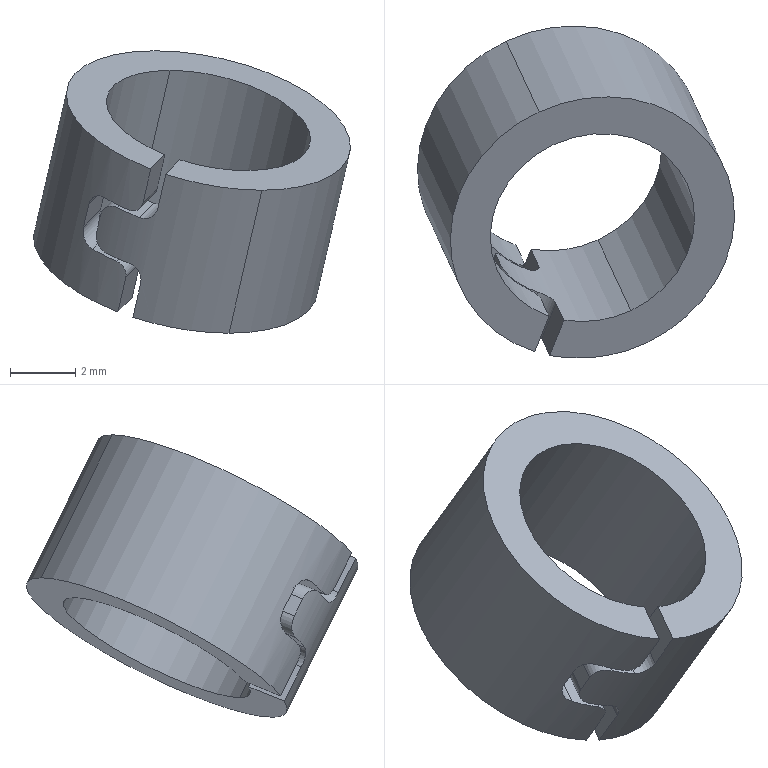Part | SolidWorks | features BaseBody 1 | 1 solid | 26 faces | box 9.725 x 10.19 x 8.66 mm | volume 146.52 mm3 | cylinder 14 | plane 12 | commonest cylinder face diameters 1 x6 6.4 x3 8.9 x3 0.8 x2
STEP:
#1=CARTESIAN_POINT('',(2002.985,-235.074,926.906));
#2=VERTEX_POINT('',#1);
#3=CARTESIAN_POINT('',(2003.992,-237.254,931.291));
#4=VERTEX_POINT('',#3);
#5=CARTESIAN_POINT('',(2003.489,-236.164,929.099));
#6=DIRECTION('',(0.2015,-0.436,0.8771));
#7=VECTOR('',#6,1000.);
#8=LINE('',#5,#7);
#9=EDGE_CURVE('',#2,#4,#8,.T.);
#10=ORIENTED_EDGE('',*,*,#9,.F.);
#11=CARTESIAN_POINT('',(1999.708,-227.989,931.181));
#12=VERTEX_POINT('',#11);
#13=CARTESIAN_POINT('',(2001.347,-231.531,929.043));
#14=DIRECTION('',(0.2015,-0.436,0.8771));
#15=DIRECTION('',(0.9077,0.4197,0.0001669));
#16=AXIS2_PLACEMENT_3D('',#13,#14,#15);
#17=CIRCLE('',#16,4.45);
#18=EDGE_CURVE('',#2,#12,#17,.T.);
#19=ORIENTED_EDGE('',*,*,#18,.T.);
#20=CARTESIAN_POINT('',(2000.715,-230.169,935.566));
#21=VERTEX_POINT('',#20);
#22=CARTESIAN_POINT('',(2000.212,-229.079,933.373));
#23=DIRECTION('',(0.2015,-0.436,0.8771));
#24=VECTOR('',#23,1000.);
#25=LINE('',#22,#24);
#26=EDGE_CURVE('',#12,#21,#25,.T.);
#27=ORIENTED_EDGE('',*,*,#26,.T.);
#28=CARTESIAN_POINT('',(2002.354,-233.711,933.429));
#29=DIRECTION('',(0.2015,-0.436,0.8771));
#30=DIRECTION('',(0.9077,0.4197,0.0001669));
#31=AXIS2_PLACEMENT_3D('',#28,#29,#30);
#32=CIRCLE('',#31,4.45);
#33=EDGE_CURVE('',#4,#21,#32,.T.);
#34=ORIENTED_EDGE('',*,*,#33,.F.);
#35=EDGE_LOOP('',(#10,#19,#27,#34));
#36=FACE_OUTER_BOUND('',#35,.T.);
#37=CARTESIAN_POINT('',(2001.85,-232.621,931.236));
#38=DIRECTION('',(0.2015,-0.436,0.8771));
#39=DIRECTION('',(-0.3682,0.7961,0.4803));
#40=AXIS2_PLACEMENT_3D('',#37,#38,#39);
#41=CYLINDRICAL_SURFACE('',#40,4.45);
#42=ADVANCED_FACE('',(#36),#41,.T.);
#43=CARTESIAN_POINT('',(2003.532,-236.259,931.892));
#44=VERTEX_POINT('',#43);
#45=CARTESIAN_POINT('',(2001.176,-231.164,934.966));
#46=VERTEX_POINT('',#45);
#47=CARTESIAN_POINT('',(2002.354,-233.711,933.429));
#48=DIRECTION('',(0.2015,-0.436,0.8771));
#49=DIRECTION('',(0.9077,0.4197,0.0001669));
#50=AXIS2_PLACEMENT_3D('',#47,#48,#49);
#51=CIRCLE('',#50,3.2);
#52=EDGE_CURVE('',#44,#46,#51,.T.);
#53=ORIENTED_EDGE('',*,*,#52,.T.);
#54=CARTESIAN_POINT('',(2000.168,-228.984,930.58));
#55=VERTEX_POINT('',#54);
#56=CARTESIAN_POINT('',(2000.672,-230.074,932.773));
#57=DIRECTION('',(0.2015,-0.436,0.8771));
#58=VECTOR('',#57,1000.);
#59=LINE('',#56,#58);
#60=EDGE_CURVE('',#55,#46,#59,.T.);
#61=ORIENTED_EDGE('',*,*,#60,.F.);
#62=CARTESIAN_POINT('',(2002.525,-234.079,927.506));
#63=VERTEX_POINT('',#62);
#64=CARTESIAN_POINT('',(2001.347,-231.531,929.043));
#65=DIRECTION('',(0.2015,-0.436,0.8771));
#66=DIRECTION('',(0.9077,0.4197,0.0001669));
#67=AXIS2_PLACEMENT_3D('',#64,#65,#66);
#68=CIRCLE('',#67,3.2);
#69=EDGE_CURVE('',#63,#55,#68,.T.);
#70=ORIENTED_EDGE('',*,*,#69,.F.);
#71=CARTESIAN_POINT('',(2003.028,-235.169,929.699));
#72=DIRECTION('',(0.2015,-0.436,0.8771));
#73=VECTOR('',#72,1000.);
#74=LINE('',#71,#73);
#75=EDGE_CURVE('',#63,#44,#74,.T.);
#76=ORIENTED_EDGE('',*,*,#75,.T.);
#77=EDGE_LOOP('',(#53,#61,#70,#76));
#78=FACE_OUTER_BOUND('',#77,.T.);
#79=CARTESIAN_POINT('',(2001.85,-232.621,931.236));
#80=DIRECTION('',(0.2015,-0.436,0.8771));
#81=DIRECTION('',(-0.3682,0.7961,0.4803));
#82=AXIS2_PLACEMENT_3D('',#79,#80,#81);
#83=CYLINDRICAL_SURFACE('',#82,3.2);
#84=ADVANCED_FACE('',(#78),#83,.F.);
#85=CARTESIAN_POINT('',(2001.043,-237.632,931.781));
#86=VERTEX_POINT('',#85);
#87=CARTESIAN_POINT('',(2002.354,-233.711,933.429));
#88=DIRECTION('',(0.2015,-0.436,0.8771));
#89=DIRECTION('',(0.9077,0.4197,0.0001669));
#90=AXIS2_PLACEMENT_3D('',#87,#88,#89);
#91=CIRCLE('',#90,4.45);
#92=EDGE_CURVE('',#86,#4,#91,.T.);
#93=ORIENTED_EDGE('',*,*,#92,.T.);
#94=ORIENTED_EDGE('',*,*,#33,.T.);
#95=CARTESIAN_POINT('',(2000.585,-237.515,931.944));
#96=VERTEX_POINT('',#95);
#97=CARTESIAN_POINT('',(2002.354,-233.711,933.429));
#98=DIRECTION('',(0.2015,-0.436,0.8771));
#99=DIRECTION('',(0.9077,0.4197,0.0001669));
#100=AXIS2_PLACEMENT_3D('',#97,#98,#99);
#101=CIRCLE('',#100,4.45);
#102=EDGE_CURVE('',#21,#96,#101,.T.);
#103=ORIENTED_EDGE('',*,*,#102,.T.);
#104=CARTESIAN_POINT('',(2001.019,-236.426,932.386));
#105=VERTEX_POINT('',#104);
#106=CARTESIAN_POINT('',(2000.802,-236.971,932.165));
#107=DIRECTION('',(-0.3465,-0.8693,-0.3525));
#108=VECTOR('',#107,1000.);
#109=LINE('',#106,#108);
#110=EDGE_CURVE('',#105,#96,#109,.T.);
#111=ORIENTED_EDGE('',*,*,#110,.F.);
#112=CARTESIAN_POINT('',(2002.354,-233.711,933.429));
#113=DIRECTION('',(0.2015,-0.436,0.8771));
#114=DIRECTION('',(0.9077,0.4197,0.0001669));
#115=AXIS2_PLACEMENT_3D('',#112,#113,#114);
#116=CIRCLE('',#115,3.2);
#117=EDGE_CURVE('',#46,#105,#116,.T.);
#118=ORIENTED_EDGE('',*,*,#117,.F.);
#119=ORIENTED_EDGE('',*,*,#52,.F.);
#120=CARTESIAN_POINT('',(2001.477,-236.543,932.223));
#121=VERTEX_POINT('',#120);
#122=CARTESIAN_POINT('',(2002.354,-233.711,933.429));
#123=DIRECTION('',(0.2015,-0.436,0.8771));
#124=DIRECTION('',(0.9077,0.4197,0.0001669));
#125=AXIS2_PLACEMENT_3D('',#122,#123,#124);
#126=CIRCLE('',#125,3.2);
#127=EDGE_CURVE('',#121,#44,#126,.T.);
#128=ORIENTED_EDGE('',*,*,#127,.F.);
#129=CARTESIAN_POINT('',(2001.26,-237.087,932.002));
#130=DIRECTION('',(-0.3465,-0.8693,-0.3525));
#131=VECTOR('',#130,1000.);
#132=LINE('',#129,#131);
#133=EDGE_CURVE('',#121,#86,#132,.T.);
#134=ORIENTED_EDGE('',*,*,#133,.T.);
#135=EDGE_LOOP('',(#93,#94,#103,#111,#118,#119,#128,#134));
#136=FACE_OUTER_BOUND('',#135,.T.);
#137=CARTESIAN_POINT('',(1956.546,-222.065,949.74));
#138=DIRECTION('',(0.2015,-0.436,0.8771));
#139=DIRECTION('',(-0.9077,-0.4197,-0.0001669));
#140=AXIS2_PLACEMENT_3D('',#137,#138,#139);
#141=PLANE('',#140);
#142=ADVANCED_FACE('',(#136),#141,.T.);
#143=CARTESIAN_POINT('',(2000.47,-234.363,927.837));
#144=VERTEX_POINT('',#143);
#145=CARTESIAN_POINT('',(2000.036,-235.452,927.395));
#146=VERTEX_POINT('',#145);
#147=CARTESIAN_POINT('',(2000.253,-234.907,927.616));
#148=DIRECTION('',(-0.3465,-0.8693,-0.3525));
#149=VECTOR('',#148,1000.);
#150=LINE('',#147,#149);
#151=EDGE_CURVE('',#144,#146,#150,.T.);
#152=ORIENTED_EDGE('',*,*,#151,.F.);
#153=CARTESIAN_POINT('',(2001.347,-231.531,929.043));
#154=DIRECTION('',(0.2015,-0.436,0.8771));
#155=DIRECTION('',(0.9077,0.4197,0.0001669));
#156=AXIS2_PLACEMENT_3D('',#153,#154,#155);
#157=CIRCLE('',#156,3.2);
#158=EDGE_CURVE('',#144,#63,#157,.T.);
#159=ORIENTED_EDGE('',*,*,#158,.T.);
#160=ORIENTED_EDGE('',*,*,#69,.T.);
#161=CARTESIAN_POINT('',(2000.012,-234.246,928.));
#162=VERTEX_POINT('',#161);
#163=CARTESIAN_POINT('',(2001.347,-231.531,929.043));
#164=DIRECTION('',(0.2015,-0.436,0.8771));
#165=DIRECTION('',(0.9077,0.4197,0.0001669));
#166=AXIS2_PLACEMENT_3D('',#163,#164,#165);
#167=CIRCLE('',#166,3.2);
#168=EDGE_CURVE('',#55,#162,#167,.T.);
#169=ORIENTED_EDGE('',*,*,#168,.T.);
#170=CARTESIAN_POINT('',(1999.578,-235.335,927.559));
#171=VERTEX_POINT('',#170);
#172=CARTESIAN_POINT('',(1999.795,-234.791,927.779));
#173=DIRECTION('',(-0.3465,-0.8693,-0.3525));
#174=VECTOR('',#173,1000.);
#175=LINE('',#172,#174);
#176=EDGE_CURVE('',#162,#171,#175,.T.);
#177=ORIENTED_EDGE('',*,*,#176,.T.);
#178=CARTESIAN_POINT('',(2001.347,-231.531,929.043));
#179=DIRECTION('',(0.2015,-0.436,0.8771));
#180=DIRECTION('',(0.9077,0.4197,0.0001669));
#181=AXIS2_PLACEMENT_3D('',#178,#179,#180);
#182=CIRCLE('',#181,4.45);
#183=EDGE_CURVE('',#12,#171,#182,.T.);
#184=ORIENTED_EDGE('',*,*,#183,.F.);
#185=ORIENTED_EDGE('',*,*,#18,.F.);
#186=CARTESIAN_POINT('',(2001.347,-231.531,929.043));
#187=DIRECTION('',(0.2015,-0.436,0.8771));
#188=DIRECTION('',(0.9077,0.4197,0.0001669));
#189=AXIS2_PLACEMENT_3D('',#186,#187,#188);
#190=CIRCLE('',#189,4.45);
#191=EDGE_CURVE('',#146,#2,#190,.T.);
#192=ORIENTED_EDGE('',*,*,#191,.F.);
#193=EDGE_LOOP('',(#152,#159,#160,#169,#177,#184,#185,#192));
#194=FACE_OUTER_BOUND('',#193,.T.);
#195=CARTESIAN_POINT('',(1955.539,-219.885,945.354));
#196=DIRECTION('',(0.2015,-0.436,0.8771));
#197=DIRECTION('',(-0.9077,-0.4197,-0.0001669));
#198=AXIS2_PLACEMENT_3D('',#195,#196,#197);
#199=PLANE('',#198);
#200=ADVANCED_FACE('',(#194),#199,.F.);
#201=CARTESIAN_POINT('',(2000.712,-234.886,928.889));
#202=VERTEX_POINT('',#201);
#203=CARTESIAN_POINT('',(2000.974,-235.453,930.03));
#204=DIRECTION('',(0.2015,-0.436,0.8771));
#205=VECTOR('',#204,1000.);
#206=LINE('',#203,#205);
#207=EDGE_CURVE('',#144,#202,#206,.T.);
#208=ORIENTED_EDGE('',*,*,#207,.T.);
#209=CARTESIAN_POINT('',(2000.354,-234.987,929.491));
#210=VERTEX_POINT('',#209);
#211=CARTESIAN_POINT('',(2000.712,-234.886,928.889));
#212=CARTESIAN_POINT('',(2000.738,-234.943,929.005));
#213=CARTESIAN_POINT('',(2000.713,-234.991,929.135));
#214=CARTESIAN_POINT('',(2000.579,-235.034,929.354));
#215=CARTESIAN_POINT('',(2000.471,-235.027,929.445));
#216=CARTESIAN_POINT('',(2000.354,-234.987,929.491));
#217=B_SPLINE_CURVE_WITH_KNOTS('',3,(#211,#212,#213,#214,#215,#216),.UNSPECIFIED.,.F.,.F.,(4,2,4),(0.,0.0003909,0.0007818),.UNSPECIFIED.);
#218=EDGE_CURVE('',#202,#210,#217,.T.);
#219=ORIENTED_EDGE('',*,*,#218,.T.);
#220=CARTESIAN_POINT('',(1999.68,-234.656,929.811));
#221=VERTEX_POINT('',#220);
#222=CARTESIAN_POINT('',(2001.689,-232.272,930.534));
#223=DIRECTION('',(-0.2015,0.436,-0.8771));
#224=DIRECTION('',(0.9077,0.4197,0.0001669));
#225=AXIS2_PLACEMENT_3D('',#222,#223,#224);
#226=CIRCLE('',#225,3.2);
#227=EDGE_CURVE('',#210,#221,#226,.T.);
#228=ORIENTED_EDGE('',*,*,#227,.T.);
#229=CARTESIAN_POINT('',(1999.4,-234.563,930.492));
#230=VERTEX_POINT('',#229);
#231=CARTESIAN_POINT('',(1999.4,-234.563,930.492));
#232=CARTESIAN_POINT('',(1999.372,-234.503,930.37));
#233=CARTESIAN_POINT('',(1999.388,-234.489,930.224));
#234=CARTESIAN_POINT('',(1999.491,-234.532,929.974));
#235=CARTESIAN_POINT('',(1999.576,-234.586,929.87));
#236=CARTESIAN_POINT('',(1999.68,-234.656,929.811));
#237=B_SPLINE_CURVE_WITH_KNOTS('',3,(#231,#232,#233,#234,#235,#236),.UNSPECIFIED.,.F.,.F.,(4,2,4),(0.,0.0004086,0.0008172),.UNSPECIFIED.);
#238=EDGE_CURVE('',#230,#221,#237,.T.);
#239=ORIENTED_EDGE('',*,*,#238,.F.);
#240=CARTESIAN_POINT('',(1999.52,-234.824,931.018));
#241=VERTEX_POINT('',#240);
#242=CARTESIAN_POINT('',(1999.46,-234.694,930.755));
#243=DIRECTION('',(0.2015,-0.436,0.8771));
#244=VECTOR('',#243,1000.);
#245=LINE('',#242,#244);
#246=EDGE_CURVE('',#230,#241,#245,.T.);
#247=ORIENTED_EDGE('',*,*,#246,.T.);
#248=CARTESIAN_POINT('',(2000.002,-235.353,931.215));
#249=VERTEX_POINT('',#248);
#250=CARTESIAN_POINT('',(1999.52,-234.824,931.018));
#251=CARTESIAN_POINT('',(1999.548,-234.885,931.139));
#252=CARTESIAN_POINT('',(1999.618,-234.986,931.223));
#253=CARTESIAN_POINT('',(1999.792,-235.185,931.288));
#254=CARTESIAN_POINT('',(1999.898,-235.283,931.273));
#255=CARTESIAN_POINT('',(2000.002,-235.353,931.215));
#256=B_SPLINE_CURVE_WITH_KNOTS('',3,(#250,#251,#252,#253,#254,#255),.UNSPECIFIED.,.F.,.F.,(4,2,4),(0.,0.0004086,0.0008172),.UNSPECIFIED.);
#257=EDGE_CURVE('',#241,#249,#256,.T.);
#258=ORIENTED_EDGE('',*,*,#257,.T.);
#259=CARTESIAN_POINT('',(2000.677,-235.685,930.895));
#260=VERTEX_POINT('',#259);
#261=CARTESIAN_POINT('',(2002.011,-232.97,931.938));
#262=DIRECTION('',(0.2015,-0.436,0.8771));
#263=DIRECTION('',(0.9077,0.4197,0.0001669));
#264=AXIS2_PLACEMENT_3D('',#261,#262,#263);
#265=CIRCLE('',#264,3.2);
#266=EDGE_CURVE('',#249,#260,#265,.T.);
#267=ORIENTED_EDGE('',*,*,#266,.T.);
#268=CARTESIAN_POINT('',(2001.236,-236.019,931.17));
#269=VERTEX_POINT('',#268);
#270=CARTESIAN_POINT('',(2001.236,-236.019,931.17));
#271=CARTESIAN_POINT('',(2001.209,-235.962,931.054));
#272=CARTESIAN_POINT('',(2001.132,-235.897,930.957));
#273=CARTESIAN_POINT('',(2000.923,-235.779,930.853));
#274=CARTESIAN_POINT('',(2000.794,-235.725,930.848));
#275=CARTESIAN_POINT('',(2000.677,-235.685,930.895));
#276=B_SPLINE_CURVE_WITH_KNOTS('',3,(#270,#271,#272,#273,#274,#275),.UNSPECIFIED.,.F.,.F.,(4,2,4),(0.,0.0003909,0.0007818),.UNSPECIFIED.);
#277=EDGE_CURVE('',#269,#260,#276,.T.);
#278=ORIENTED_EDGE('',*,*,#277,.F.);
#279=CARTESIAN_POINT('',(2000.974,-235.453,930.03));
#280=DIRECTION('',(0.2015,-0.436,0.8771));
#281=VECTOR('',#280,1000.);
#282=LINE('',#279,#281);
#283=EDGE_CURVE('',#269,#121,#282,.T.);
#284=ORIENTED_EDGE('',*,*,#283,.T.);
#285=ORIENTED_EDGE('',*,*,#127,.T.);
#286=ORIENTED_EDGE('',*,*,#75,.F.);
#287=ORIENTED_EDGE('',*,*,#158,.F.);
#288=EDGE_LOOP('',(#208,#219,#228,#239,#247,#258,#267,#278,#284,#285,#286,#287));
#289=FACE_OUTER_BOUND('',#288,.T.);
#290=CARTESIAN_POINT('',(2001.85,-232.621,931.236));
#291=DIRECTION('',(0.2015,-0.436,0.8771));
#292=DIRECTION('',(-0.3682,0.7961,0.4803));
#293=AXIS2_PLACEMENT_3D('',#290,#291,#292);
#294=CYLINDRICAL_SURFACE('',#293,3.2);
#295=ADVANCED_FACE('',(#289),#294,.F.);
#296=CARTESIAN_POINT('',(2000.778,-235.903,931.333));
#297=VERTEX_POINT('',#296);
#298=CARTESIAN_POINT('',(2000.516,-235.336,930.193));
#299=DIRECTION('',(-0.2015,0.436,-0.8771));
#300=VECTOR('',#299,1000.);
#301=LINE('',#298,#300);
#302=EDGE_CURVE('',#105,#297,#301,.T.);
#303=ORIENTED_EDGE('',*,*,#302,.T.);
#304=CARTESIAN_POINT('',(2000.35,-235.586,931.133));
#305=VERTEX_POINT('',#304);
#306=CARTESIAN_POINT('',(2000.778,-235.903,931.333));
#307=CARTESIAN_POINT('',(2000.756,-235.857,931.24));
#308=CARTESIAN_POINT('',(2000.696,-235.799,931.164));
#309=CARTESIAN_POINT('',(2000.536,-235.685,931.089));
#310=CARTESIAN_POINT('',(2000.438,-235.629,931.091));
#311=CARTESIAN_POINT('',(2000.35,-235.586,931.133));
#312=B_SPLINE_CURVE_WITH_KNOTS('',3,(#306,#307,#308,#309,#310,#311),.UNSPECIFIED.,.F.,.F.,(4,2,4),(0.,0.0003145,0.0006289),.UNSPECIFIED.);
#313=EDGE_CURVE('',#297,#305,#312,.T.);
#314=ORIENTED_EDGE('',*,*,#313,.T.);
#315=CARTESIAN_POINT('',(1999.641,-235.086,931.544));
#316=VERTEX_POINT('',#315);
#317=CARTESIAN_POINT('',(2002.032,-233.014,932.025));
#318=DIRECTION('',(-0.2015,0.436,-0.8771));
#319=DIRECTION('',(0.9077,0.4197,0.0001669));
#320=AXIS2_PLACEMENT_3D('',#317,#318,#319);
#321=CIRCLE('',#320,3.2);
#322=EDGE_CURVE('',#305,#316,#321,.T.);
#323=ORIENTED_EDGE('',*,*,#322,.T.);
#324=CARTESIAN_POINT('',(1999.201,-234.454,931.389));
#325=VERTEX_POINT('',#324);
#326=CARTESIAN_POINT('',(1999.201,-234.454,931.389));
#327=CARTESIAN_POINT('',(1999.216,-234.486,931.453));
#328=CARTESIAN_POINT('',(1999.24,-234.533,931.506));
#329=CARTESIAN_POINT('',(1999.302,-234.64,931.58));
#330=CARTESIAN_POINT('',(1999.338,-234.7,931.604));
#331=CARTESIAN_POINT('',(1999.457,-234.878,931.636));
#332=CARTESIAN_POINT('',(1999.549,-234.995,931.61));
#333=CARTESIAN_POINT('',(1999.641,-235.086,931.544));
#334=B_SPLINE_CURVE_WITH_KNOTS('',3,(#326,#327,#328,#329,#330,#331,#332,#333),.UNSPECIFIED.,.F.,.F.,(4,2,2,4),(0.,0.0002158,0.0004316,0.0008631),.UNSPECIFIED.);
#335=EDGE_CURVE('',#325,#316,#334,.T.);
#336=ORIENTED_EDGE('',*,*,#335,.F.);
#337=CARTESIAN_POINT('',(1999.04,-234.105,930.688));
#338=VERTEX_POINT('',#337);
#339=CARTESIAN_POINT('',(1999.121,-234.28,931.039));
#340=DIRECTION('',(-0.2015,0.436,-0.8771));
#341=VECTOR('',#340,1000.);
#342=LINE('',#339,#341);
#343=EDGE_CURVE('',#325,#338,#342,.T.);
#344=ORIENTED_EDGE('',*,*,#343,.T.);
#345=CARTESIAN_POINT('',(1999.279,-234.301,929.965));
#346=VERTEX_POINT('',#345);
#347=CARTESIAN_POINT('',(1999.04,-234.105,930.688));
#348=CARTESIAN_POINT('',(1999.025,-234.073,930.624));
#349=CARTESIAN_POINT('',(1999.021,-234.058,930.551));
#350=CARTESIAN_POINT('',(1999.032,-234.057,930.407));
#351=CARTESIAN_POINT('',(1999.047,-234.07,930.336));
#352=CARTESIAN_POINT('',(1999.113,-234.134,930.14));
#353=CARTESIAN_POINT('',(1999.187,-234.21,930.032));
#354=CARTESIAN_POINT('',(1999.279,-234.301,929.965));
#355=B_SPLINE_CURVE_WITH_KNOTS('',3,(#347,#348,#349,#350,#351,#352,#353,#354),.UNSPECIFIED.,.F.,.F.,(4,2,2,4),(0.,0.0002158,0.0004316,0.0008631),.UNSPECIFIED.);
#356=EDGE_CURVE('',#338,#346,#355,.T.);
#357=ORIENTED_EDGE('',*,*,#356,.T.);
#358=CARTESIAN_POINT('',(1999.987,-234.801,929.554));
#359=VERTEX_POINT('',#358);
#360=CARTESIAN_POINT('',(2001.669,-232.229,930.447));
#361=DIRECTION('',(0.2015,-0.436,0.8771));
#362=DIRECTION('',(0.9077,0.4197,0.0001669));
#363=AXIS2_PLACEMENT_3D('',#360,#361,#362);
#364=CIRCLE('',#363,3.2);
#365=EDGE_CURVE('',#346,#359,#364,.T.);
#366=ORIENTED_EDGE('',*,*,#365,.T.);
#367=CARTESIAN_POINT('',(2000.254,-234.769,929.053));
#368=VERTEX_POINT('',#367);
#369=CARTESIAN_POINT('',(2000.254,-234.769,929.053));
#370=CARTESIAN_POINT('',(2000.275,-234.816,929.146));
#371=CARTESIAN_POINT('',(2000.257,-234.848,929.252));
#372=CARTESIAN_POINT('',(2000.156,-234.863,929.436));
#373=CARTESIAN_POINT('',(2000.075,-234.844,929.513));
#374=CARTESIAN_POINT('',(1999.987,-234.801,929.554));
#375=B_SPLINE_CURVE_WITH_KNOTS('',3,(#369,#370,#371,#372,#373,#374),.UNSPECIFIED.,.F.,.F.,(4,2,4),(0.,0.0003145,0.0006289),.UNSPECIFIED.);
#376=EDGE_CURVE('',#368,#359,#375,.T.);
#377=ORIENTED_EDGE('',*,*,#376,.F.);
#378=CARTESIAN_POINT('',(2000.516,-235.336,930.193));
#379=DIRECTION('',(-0.2015,0.436,-0.8771));
#380=VECTOR('',#379,1000.);
#381=LINE('',#378,#380);
#382=EDGE_CURVE('',#368,#162,#381,.T.);
#383=ORIENTED_EDGE('',*,*,#382,.T.);
#384=ORIENTED_EDGE('',*,*,#168,.F.);
#385=ORIENTED_EDGE('',*,*,#60,.T.);
#386=ORIENTED_EDGE('',*,*,#117,.T.);
#387=EDGE_LOOP('',(#303,#314,#323,#336,#344,#357,#366,#377,#383,#384,#385,#386));
#388=FACE_OUTER_BOUND('',#387,.T.);
#389=CARTESIAN_POINT('',(2001.85,-232.621,931.236));
#390=DIRECTION('',(0.2015,-0.436,0.8771));
#391=DIRECTION('',(-0.3682,0.7961,0.4803));
#392=AXIS2_PLACEMENT_3D('',#389,#390,#391);
#393=CYLINDRICAL_SURFACE('',#392,3.2);
#394=ADVANCED_FACE('',(#388),#393,.F.);
#395=ORIENTED_EDGE('',*,*,#191,.T.);
#396=ORIENTED_EDGE('',*,*,#9,.T.);
#397=ORIENTED_EDGE('',*,*,#92,.F.);
#398=CARTESIAN_POINT('',(2000.802,-237.108,930.729));
#399=VERTEX_POINT('',#398);
#400=CARTESIAN_POINT('',(2000.54,-236.542,929.588));
#401=DIRECTION('',(0.2015,-0.436,0.8771));
#402=VECTOR('',#401,1000.);
#403=LINE('',#400,#402);
#404=EDGE_CURVE('',#399,#86,#403,.T.);
#405=ORIENTED_EDGE('',*,*,#404,.F.);
#406=CARTESIAN_POINT('',(2000.243,-236.774,930.453));
#407=VERTEX_POINT('',#406);
#408=CARTESIAN_POINT('',(2000.802,-237.108,930.729));
#409=CARTESIAN_POINT('',(2000.775,-237.051,930.613));
#410=CARTESIAN_POINT('',(2000.698,-236.985,930.516));
#411=CARTESIAN_POINT('',(2000.49,-236.865,930.413));
#412=CARTESIAN_POINT('',(2000.361,-236.811,930.407));
#413=CARTESIAN_POINT('',(2000.243,-236.774,930.453));
#414=B_SPLINE_CURVE_WITH_KNOTS('',3,(#408,#409,#410,#411,#412,#413),.UNSPECIFIED.,.F.,.F.,(4,2,4),(0.,0.0003908,0.0007816),.UNSPECIFIED.);
#415=EDGE_CURVE('',#399,#407,#414,.T.);
#416=ORIENTED_EDGE('',*,*,#415,.T.);
#417=CARTESIAN_POINT('',(1999.551,-236.485,930.756));
#418=VERTEX_POINT('',#417);
#419=CARTESIAN_POINT('',(2002.011,-232.97,931.938));
#420=DIRECTION('',(0.2015,-0.436,0.8771));
#421=DIRECTION('',(0.9077,0.4197,0.0001669));
#422=AXIS2_PLACEMENT_3D('',#419,#420,#421);
#423=CIRCLE('',#422,4.45);
#424=EDGE_CURVE('',#418,#407,#423,.T.);
#425=ORIENTED_EDGE('',*,*,#424,.F.);
#426=CARTESIAN_POINT('',(1999.045,-236.017,930.534));
#427=VERTEX_POINT('',#426);
#428=CARTESIAN_POINT('',(1999.045,-236.017,930.534));
#429=CARTESIAN_POINT('',(1999.072,-236.076,930.653));
#430=CARTESIAN_POINT('',(1999.143,-236.165,930.741));
#431=CARTESIAN_POINT('',(1999.328,-236.341,930.818));
#432=CARTESIAN_POINT('',(1999.442,-236.426,930.81));
#433=CARTESIAN_POINT('',(1999.551,-236.485,930.756));
#434=B_SPLINE_CURVE_WITH_KNOTS('',3,(#428,#429,#430,#431,#432,#433),.UNSPECIFIED.,.F.,.F.,(4,2,4),(0.,0.0003993,0.0007985),.UNSPECIFIED.);
#435=EDGE_CURVE('',#427,#418,#434,.T.);
#436=ORIENTED_EDGE('',*,*,#435,.F.);
#437=CARTESIAN_POINT('',(1998.924,-235.755,930.008));
#438=VERTEX_POINT('',#437);
#439=CARTESIAN_POINT('',(1998.985,-235.886,930.271));
#440=DIRECTION('',(0.2015,-0.436,0.8771));
#441=VECTOR('',#440,1000.);
#442=LINE('',#439,#441);
#443=EDGE_CURVE('',#438,#427,#442,.T.);
#444=ORIENTED_EDGE('',*,*,#443,.F.);
#445=CARTESIAN_POINT('',(1999.229,-235.787,929.352));
#446=VERTEX_POINT('',#445);
#447=CARTESIAN_POINT('',(1998.924,-235.755,930.008));
#448=CARTESIAN_POINT('',(1998.897,-235.697,929.89));
#449=CARTESIAN_POINT('',(1998.915,-235.672,929.749));
#450=CARTESIAN_POINT('',(1999.027,-235.689,929.508));
#451=CARTESIAN_POINT('',(1999.12,-235.729,929.406));
#452=CARTESIAN_POINT('',(1999.229,-235.787,929.352));
#453=B_SPLINE_CURVE_WITH_KNOTS('',3,(#447,#448,#449,#450,#451,#452),.UNSPECIFIED.,.F.,.F.,(4,2,4),(0.,0.0003993,0.0007985),.UNSPECIFIED.);
#454=EDGE_CURVE('',#438,#446,#453,.T.);
#455=ORIENTED_EDGE('',*,*,#454,.T.);
#456=CARTESIAN_POINT('',(1999.92,-236.076,929.05));
#457=VERTEX_POINT('',#456);
#458=CARTESIAN_POINT('',(2001.689,-232.272,930.534));
#459=DIRECTION('',(-0.2015,0.436,-0.8771));
#460=DIRECTION('',(0.9077,0.4197,0.0001669));
#461=AXIS2_PLACEMENT_3D('',#458,#459,#460);
#462=CIRCLE('',#461,4.45);
#463=EDGE_CURVE('',#457,#446,#462,.T.);
#464=ORIENTED_EDGE('',*,*,#463,.F.);
#465=CARTESIAN_POINT('',(2000.278,-235.975,928.448));
#466=VERTEX_POINT('',#465);
#467=CARTESIAN_POINT('',(2000.278,-235.975,928.448));
#468=CARTESIAN_POINT('',(2000.304,-236.032,928.564));
#469=CARTESIAN_POINT('',(2000.279,-236.079,928.693));
#470=CARTESIAN_POINT('',(2000.146,-236.12,928.914));
#471=CARTESIAN_POINT('',(2000.038,-236.113,929.004));
#472=CARTESIAN_POINT('',(1999.92,-236.076,929.05));
#473=B_SPLINE_CURVE_WITH_KNOTS('',3,(#467,#468,#469,#470,#471,#472),.UNSPECIFIED.,.F.,.F.,(4,2,4),(0.,0.0003908,0.0007816),.UNSPECIFIED.);
#474=EDGE_CURVE('',#466,#457,#473,.T.);
#475=ORIENTED_EDGE('',*,*,#474,.F.);
#476=CARTESIAN_POINT('',(2000.54,-236.542,929.588));
#477=DIRECTION('',(0.2015,-0.436,0.8771));
#478=VECTOR('',#477,1000.);
#479=LINE('',#476,#478);
#480=EDGE_CURVE('',#146,#466,#479,.T.);
#481=ORIENTED_EDGE('',*,*,#480,.F.);
#482=EDGE_LOOP('',(#395,#396,#397,#405,#416,#425,#436,#444,#455,#464,#475,#481));
#483=FACE_OUTER_BOUND('',#482,.T.);
#484=CARTESIAN_POINT('',(2001.85,-232.621,931.236));
#485=DIRECTION('',(0.2015,-0.436,0.8771));
#486=DIRECTION('',(-0.3682,0.7961,0.4803));
#487=AXIS2_PLACEMENT_3D('',#484,#485,#486);
#488=CYLINDRICAL_SURFACE('',#487,4.45);
#489=ADVANCED_FACE('',(#483),#488,.T.);
#490=ORIENTED_EDGE('',*,*,#102,.F.);
#491=ORIENTED_EDGE('',*,*,#26,.F.);
#492=ORIENTED_EDGE('',*,*,#183,.T.);
#493=CARTESIAN_POINT('',(1999.82,-235.858,928.611));
#494=VERTEX_POINT('',#493);
#495=CARTESIAN_POINT('',(2000.082,-236.425,929.751));
#496=DIRECTION('',(0.2015,-0.436,0.8771));
#497=VECTOR('',#496,1000.);
#498=LINE('',#495,#497);
#499=EDGE_CURVE('',#171,#494,#498,.T.);
#500=ORIENTED_EDGE('',*,*,#499,.T.);
#501=CARTESIAN_POINT('',(1999.548,-235.904,929.107));
#502=VERTEX_POINT('',#501);
#503=CARTESIAN_POINT('',(1999.82,-235.858,928.611));
#504=CARTESIAN_POINT('',(1999.841,-235.904,928.704));
#505=CARTESIAN_POINT('',(1999.823,-235.938,928.81));
#506=CARTESIAN_POINT('',(1999.721,-235.957,928.992));
#507=CARTESIAN_POINT('',(1999.638,-235.942,929.067));
#508=CARTESIAN_POINT('',(1999.548,-235.904,929.107));
#509=B_SPLINE_CURVE_WITH_KNOTS('',3,(#503,#504,#505,#506,#507,#508),.UNSPECIFIED.,.F.,.F.,(4,2,4),(0.,0.0003135,0.0006271),.UNSPECIFIED.);
#510=EDGE_CURVE('',#494,#502,#509,.T.);
#511=ORIENTED_EDGE('',*,*,#510,.T.);
#512=CARTESIAN_POINT('',(1998.804,-235.494,929.482));
#513=VERTEX_POINT('',#512);
#514=CARTESIAN_POINT('',(2001.669,-232.229,930.447));
#515=DIRECTION('',(0.2015,-0.436,0.8771));
#516=DIRECTION('',(0.9077,0.4197,0.0001669));
#517=AXIS2_PLACEMENT_3D('',#514,#515,#516);
#518=CIRCLE('',#517,4.45);
#519=EDGE_CURVE('',#513,#502,#518,.T.);
#520=ORIENTED_EDGE('',*,*,#519,.F.);
#521=CARTESIAN_POINT('',(1998.523,-235.403,930.162));
#522=VERTEX_POINT('',#521);
#523=CARTESIAN_POINT('',(1998.523,-235.403,930.162));
#524=CARTESIAN_POINT('',(1998.495,-235.342,930.04));
#525=CARTESIAN_POINT('',(1998.512,-235.327,929.894));
#526=CARTESIAN_POINT('',(1998.616,-235.368,929.645));
#527=CARTESIAN_POINT('',(1998.702,-235.422,929.541));
#528=CARTESIAN_POINT('',(1998.804,-235.494,929.482));
#529=B_SPLINE_CURVE_WITH_KNOTS('',3,(#523,#524,#525,#526,#527,#528),.UNSPECIFIED.,.F.,.F.,(4,2,4),(0.,0.0004086,0.0008171),.UNSPECIFIED.);
#530=EDGE_CURVE('',#522,#513,#529,.T.);
#531=ORIENTED_EDGE('',*,*,#530,.F.);
#532=CARTESIAN_POINT('',(1998.684,-235.751,930.863));
#533=VERTEX_POINT('',#532);
#534=CARTESIAN_POINT('',(1998.603,-235.577,930.512));
#535=DIRECTION('',(-0.2015,0.436,-0.8771));
#536=VECTOR('',#535,1000.);
#537=LINE('',#534,#536);
#538=EDGE_CURVE('',#533,#522,#537,.T.);
#539=ORIENTED_EDGE('',*,*,#538,.F.);
#540=CARTESIAN_POINT('',(1999.166,-236.279,931.06));
#541=VERTEX_POINT('',#540);
#542=CARTESIAN_POINT('',(1998.684,-235.751,930.863));
#543=CARTESIAN_POINT('',(1998.712,-235.812,930.984));
#544=CARTESIAN_POINT('',(1998.782,-235.911,931.069));
#545=CARTESIAN_POINT('',(1998.958,-236.109,931.135));
#546=CARTESIAN_POINT('',(1999.064,-236.207,931.12));
#547=CARTESIAN_POINT('',(1999.166,-236.279,931.06));
#548=B_SPLINE_CURVE_WITH_KNOTS('',3,(#542,#543,#544,#545,#546,#547),.UNSPECIFIED.,.F.,.F.,(4,2,4),(0.,0.0004086,0.0008171),.UNSPECIFIED.);
#549=EDGE_CURVE('',#533,#541,#548,.T.);
#550=ORIENTED_EDGE('',*,*,#549,.T.);
#551=CARTESIAN_POINT('',(1999.91,-236.689,930.686));
#552=VERTEX_POINT('',#551);
#553=CARTESIAN_POINT('',(2002.032,-233.014,932.025));
#554=DIRECTION('',(-0.2015,0.436,-0.8771));
#555=DIRECTION('',(0.9077,0.4197,0.0001669));
#556=AXIS2_PLACEMENT_3D('',#553,#554,#555);
#557=CIRCLE('',#556,4.45);
#558=EDGE_CURVE('',#552,#541,#557,.T.);
#559=ORIENTED_EDGE('',*,*,#558,.F.);
#560=CARTESIAN_POINT('',(2000.343,-236.992,930.892));
#561=VERTEX_POINT('',#560);
#562=CARTESIAN_POINT('',(2000.343,-236.992,930.892));
#563=CARTESIAN_POINT('',(2000.322,-236.946,930.799));
#564=CARTESIAN_POINT('',(2000.262,-236.889,930.723));
#565=CARTESIAN_POINT('',(2000.101,-236.779,930.646));
#566=CARTESIAN_POINT('',(2000.001,-236.727,930.646));
#567=CARTESIAN_POINT('',(1999.91,-236.689,930.686));
#568=B_SPLINE_CURVE_WITH_KNOTS('',3,(#562,#563,#564,#565,#566,#567),.UNSPECIFIED.,.F.,.F.,(4,2,4),(0.,0.0003135,0.0006271),.UNSPECIFIED.);
#569=EDGE_CURVE('',#561,#552,#568,.T.);
#570=ORIENTED_EDGE('',*,*,#569,.F.);
#571=CARTESIAN_POINT('',(2000.082,-236.425,929.751));
#572=DIRECTION('',(-0.2015,0.436,-0.8771));
#573=VECTOR('',#572,1000.);
#574=LINE('',#571,#573);
#575=EDGE_CURVE('',#96,#561,#574,.T.);
#576=ORIENTED_EDGE('',*,*,#575,.F.);
#577=EDGE_LOOP('',(#490,#491,#492,#500,#511,#520,#531,#539,#550,#559,#570,#576));
#578=FACE_OUTER_BOUND('',#577,.T.);
#579=CARTESIAN_POINT('',(2001.85,-232.621,931.236));
#580=DIRECTION('',(0.2015,-0.436,0.8771));
#581=DIRECTION('',(-0.3682,0.7961,0.4803));
#582=AXIS2_PLACEMENT_3D('',#579,#580,#581);
#583=CYLINDRICAL_SURFACE('',#582,4.45);
#584=ADVANCED_FACE('',(#578),#583,.T.);
#585=CARTESIAN_POINT('',(2001.019,-236.564,930.949));
#586=DIRECTION('',(-0.3465,-0.8693,-0.3525));
#587=VECTOR('',#586,1000.);
#588=LINE('',#585,#587);
#589=EDGE_CURVE('',#269,#399,#588,.T.);
#590=ORIENTED_EDGE('',*,*,#589,.T.);
#591=ORIENTED_EDGE('',*,*,#404,.T.);
#592=ORIENTED_EDGE('',*,*,#133,.F.);
#593=ORIENTED_EDGE('',*,*,#283,.F.);
#594=EDGE_LOOP('',(#590,#591,#592,#593));
#595=FACE_OUTER_BOUND('',#594,.T.);
#596=CARTESIAN_POINT('',(2001.576,-231.589,928.962));
#597=DIRECTION('',(0.9161,-0.2329,-0.3262));
#598=DIRECTION('',(-0.2015,0.436,-0.8771));
#599=AXIS2_PLACEMENT_3D('',#596,#597,#598);
#600=PLANE('',#599);
#601=ADVANCED_FACE('',(#595),#600,.F.);
#602=CARTESIAN_POINT('',(2001.002,-234.868,931.226));
#603=DIRECTION('',(-0.3465,-0.8693,-0.3525));
#604=VECTOR('',#603,1000.);
#605=LINE('',#602,#604);
#606=EDGE_CURVE('',#260,#407,#605,.T.);
#607=ORIENTED_EDGE('',*,*,#606,.T.);
#608=ORIENTED_EDGE('',*,*,#415,.F.);
#609=ORIENTED_EDGE('',*,*,#589,.F.);
#610=ORIENTED_EDGE('',*,*,#277,.T.);
#611=EDGE_LOOP('',(#607,#608,#609,#610));
#612=FACE_OUTER_BOUND('',#611,.T.);
#613=CARTESIAN_POINT('',(2001.103,-235.086,931.665));
#614=DIRECTION('',(-0.3465,-0.8693,-0.3525));
#615=DIRECTION('',(0.2015,-0.436,0.8771));
#616=AXIS2_PLACEMENT_3D('',#613,#614,#615);
#617=CYLINDRICAL_SURFACE('',#616,0.5002);
#618=ADVANCED_FACE('',(#612),#617,.F.);
#619=ORIENTED_EDGE('',*,*,#266,.F.);
#620=CARTESIAN_POINT('',(1999.777,-235.919,930.985));
#621=DIRECTION('',(-0.3465,-0.8693,-0.3525));
#622=VECTOR('',#621,1000.);
#623=LINE('',#620,#622);
#624=EDGE_CURVE('',#249,#418,#623,.T.);
#625=ORIENTED_EDGE('',*,*,#624,.T.);
#626=ORIENTED_EDGE('',*,*,#424,.T.);
#627=ORIENTED_EDGE('',*,*,#606,.F.);
#628=EDGE_LOOP('',(#619,#625,#626,#627));
#629=FACE_OUTER_BOUND('',#628,.T.);
#630=CARTESIAN_POINT('',(1915.801,-250.201,943.174));
#631=DIRECTION('',(0.2015,-0.436,0.8771));
#632=DIRECTION('',(-0.8093,-0.5785,-0.1017));
#633=AXIS2_PLACEMENT_3D('',#630,#631,#632);
#634=PLANE('',#633);
#635=ADVANCED_FACE('',(#629),#634,.T.);
#636=ORIENTED_EDGE('',*,*,#257,.F.);
#637=CARTESIAN_POINT('',(1999.711,-234.347,931.211));
#638=DIRECTION('',(-0.3465,-0.8693,-0.3525));
#639=VECTOR('',#638,1000.);
#640=LINE('',#637,#639);
#641=EDGE_CURVE('',#241,#427,#640,.T.);
#642=ORIENTED_EDGE('',*,*,#641,.T.);
#643=ORIENTED_EDGE('',*,*,#435,.T.);
#644=ORIENTED_EDGE('',*,*,#624,.F.);
#645=EDGE_LOOP('',(#636,#642,#643,#644));
#646=FACE_OUTER_BOUND('',#645,.T.);
#647=CARTESIAN_POINT('',(2000.169,-234.463,931.048));
#648=DIRECTION('',(-0.3465,-0.8693,-0.3525));
#649=DIRECTION('',(-0.2015,0.436,-0.8771));
#650=AXIS2_PLACEMENT_3D('',#647,#648,#649);
#651=CYLINDRICAL_SURFACE('',#650,0.5002);
#652=ADVANCED_FACE('',(#646),#651,.T.);
#653=CARTESIAN_POINT('',(1999.162,-235.159,930.25));
#654=DIRECTION('',(-0.3465,-0.8693,-0.3525));
#655=VECTOR('',#654,1000.);
#656=LINE('',#653,#655);
#657=EDGE_CURVE('',#230,#438,#656,.T.);
#658=ORIENTED_EDGE('',*,*,#657,.T.);
#659=ORIENTED_EDGE('',*,*,#443,.T.);
#660=ORIENTED_EDGE('',*,*,#641,.F.);
#661=ORIENTED_EDGE('',*,*,#246,.F.);
#662=EDGE_LOOP('',(#658,#659,#660,#661));
#663=FACE_OUTER_BOUND('',#662,.T.);
#664=CARTESIAN_POINT('',(2000.37,-232.129,931.479));
#665=DIRECTION('',(0.9161,-0.2329,-0.3262));
#666=DIRECTION('',(-0.2015,0.436,-0.8771));
#667=AXIS2_PLACEMENT_3D('',#664,#665,#666);
#668=PLANE('',#667);
#669=ADVANCED_FACE('',(#663),#668,.F.);
#670=ORIENTED_EDGE('',*,*,#238,.T.);
#671=CARTESIAN_POINT('',(1999.948,-233.984,930.084));
#672=DIRECTION('',(-0.3465,-0.8693,-0.3525));
#673=VECTOR('',#672,1000.);
#674=LINE('',#671,#673);
#675=EDGE_CURVE('',#221,#446,#674,.T.);
#676=ORIENTED_EDGE('',*,*,#675,.T.);
#677=ORIENTED_EDGE('',*,*,#454,.F.);
#678=ORIENTED_EDGE('',*,*,#657,.F.);
#679=EDGE_LOOP('',(#670,#676,#677,#678));
#680=FACE_OUTER_BOUND('',#679,.T.);
#681=CARTESIAN_POINT('',(2000.048,-234.202,930.522));
#682=DIRECTION('',(-0.3465,-0.8693,-0.3525));
#683=DIRECTION('',(0.9161,-0.2329,-0.3262));
#684=AXIS2_PLACEMENT_3D('',#681,#682,#683);
#685=CYLINDRICAL_SURFACE('',#684,0.5002);
#686=ADVANCED_FACE('',(#680),#685,.T.);
#687=ORIENTED_EDGE('',*,*,#227,.F.);
#688=CARTESIAN_POINT('',(2000.137,-235.532,929.271));
#689=DIRECTION('',(-0.3465,-0.8693,-0.3525));
#690=VECTOR('',#689,1000.);
#691=LINE('',#688,#690);
#692=EDGE_CURVE('',#210,#457,#691,.T.);
#693=ORIENTED_EDGE('',*,*,#692,.T.);
#694=ORIENTED_EDGE('',*,*,#463,.T.);
#695=ORIENTED_EDGE('',*,*,#675,.F.);
#696=EDGE_LOOP('',(#687,#693,#694,#695));
#697=FACE_OUTER_BOUND('',#696,.T.);
#698=CARTESIAN_POINT('',(1916.126,-249.041,941.852));
#699=DIRECTION('',(-0.2015,0.436,-0.8771));
#700=DIRECTION('',(0.8093,0.5785,0.1017));
#701=AXIS2_PLACEMENT_3D('',#698,#699,#700);
#702=PLANE('',#701);
#703=ADVANCED_FACE('',(#697),#702,.T.);
#704=CARTESIAN_POINT('',(2001.038,-234.068,929.221));
#705=DIRECTION('',(-0.3465,-0.8693,-0.3525));
#706=VECTOR('',#705,1000.);
#707=LINE('',#704,#706);
#708=EDGE_CURVE('',#202,#466,#707,.T.);
#709=ORIENTED_EDGE('',*,*,#708,.T.);
#710=ORIENTED_EDGE('',*,*,#474,.T.);
#711=ORIENTED_EDGE('',*,*,#692,.F.);
#712=ORIENTED_EDGE('',*,*,#218,.F.);
#713=EDGE_LOOP('',(#709,#710,#711,#712));
#714=FACE_OUTER_BOUND('',#713,.T.);
#715=CARTESIAN_POINT('',(2000.579,-233.952,929.384));
#716=DIRECTION('',(-0.3465,-0.8693,-0.3525));
#717=DIRECTION('',(-0.9161,0.2329,0.3262));
#718=AXIS2_PLACEMENT_3D('',#715,#716,#717);
#719=CYLINDRICAL_SURFACE('',#718,0.5002);
#720=ADVANCED_FACE('',(#714),#719,.F.);
#721=ORIENTED_EDGE('',*,*,#151,.T.);
#722=ORIENTED_EDGE('',*,*,#480,.T.);
#723=ORIENTED_EDGE('',*,*,#708,.F.);
#724=ORIENTED_EDGE('',*,*,#207,.F.);
#725=EDGE_LOOP('',(#721,#722,#723,#724));
#726=FACE_OUTER_BOUND('',#725,.T.);
#727=CARTESIAN_POINT('',(2001.576,-231.589,928.962));
#728=DIRECTION('',(0.9161,-0.2329,-0.3262));
#729=DIRECTION('',(-0.2015,0.436,-0.8771));
#730=AXIS2_PLACEMENT_3D('',#727,#728,#729);
#731=PLANE('',#730);
#732=ADVANCED_FACE('',(#726),#731,.F.);
#733=CARTESIAN_POINT('',(2000.037,-235.314,928.832));
#734=DIRECTION('',(-0.3465,-0.8693,-0.3525));
#735=VECTOR('',#734,1000.);
#736=LINE('',#733,#735);
#737=EDGE_CURVE('',#368,#494,#736,.T.);
#738=ORIENTED_EDGE('',*,*,#737,.T.);
#739=ORIENTED_EDGE('',*,*,#499,.F.);
#740=ORIENTED_EDGE('',*,*,#176,.F.);
#741=ORIENTED_EDGE('',*,*,#382,.F.);
#742=EDGE_LOOP('',(#738,#739,#740,#741));
#743=FACE_OUTER_BOUND('',#742,.T.);
#744=CARTESIAN_POINT('',(2002.125,-233.653,933.51));
#745=DIRECTION('',(-0.9161,0.2329,0.3262));
#746=DIRECTION('',(0.2015,-0.436,0.8771));
#747=AXIS2_PLACEMENT_3D('',#744,#745,#746);
#748=PLANE('',#747);
#749=ADVANCED_FACE('',(#743),#748,.F.);
#750=ORIENTED_EDGE('',*,*,#376,.T.);
#751=CARTESIAN_POINT('',(2000.294,-234.033,929.866));
#752=DIRECTION('',(-0.3465,-0.8693,-0.3525));
#753=VECTOR('',#752,1000.);
#754=LINE('',#751,#753);
#755=EDGE_CURVE('',#359,#502,#754,.T.);
#756=ORIENTED_EDGE('',*,*,#755,.T.);
#757=ORIENTED_EDGE('',*,*,#510,.F.);
#758=ORIENTED_EDGE('',*,*,#737,.F.);
#759=EDGE_LOOP('',(#750,#756,#757,#758));
#760=FACE_OUTER_BOUND('',#759,.T.);
#761=CARTESIAN_POINT('',(2000.213,-233.859,929.515));
#762=DIRECTION('',(-0.3465,-0.8693,-0.3525));
#763=DIRECTION('',(-0.9161,0.2329,0.3262));
#764=AXIS2_PLACEMENT_3D('',#761,#762,#763);
#765=CYLINDRICAL_SURFACE('',#764,0.4002);
#766=ADVANCED_FACE('',(#760),#765,.T.);
#767=ORIENTED_EDGE('',*,*,#365,.F.);
#768=CARTESIAN_POINT('',(1999.041,-234.898,929.723));
#769=DIRECTION('',(-0.3465,-0.8693,-0.3525));
#770=VECTOR('',#769,1000.);
#771=LINE('',#768,#770);
#772=EDGE_CURVE('',#346,#513,#771,.T.);
#773=ORIENTED_EDGE('',*,*,#772,.T.);
#774=ORIENTED_EDGE('',*,*,#519,.T.);
#775=ORIENTED_EDGE('',*,*,#755,.F.);
#776=EDGE_LOOP('',(#767,#773,#774,#775));
#777=FACE_OUTER_BOUND('',#776,.T.);
#778=CARTESIAN_POINT('',(1915.054,-249.749,941.632));
#779=DIRECTION('',(0.2015,-0.436,0.8771));
#780=DIRECTION('',(-0.8093,-0.5785,-0.1017));
#781=AXIS2_PLACEMENT_3D('',#778,#779,#780);
#782=PLANE('',#781);
#783=ADVANCED_FACE('',(#777),#782,.T.);
#784=CARTESIAN_POINT('',(1999.112,-233.925,930.761));
#785=DIRECTION('',(-0.3465,-0.8693,-0.3525));
#786=VECTOR('',#785,1000.);
#787=LINE('',#784,#786);
#788=EDGE_CURVE('',#338,#522,#787,.T.);
#789=ORIENTED_EDGE('',*,*,#788,.T.);
#790=ORIENTED_EDGE('',*,*,#530,.T.);
#791=ORIENTED_EDGE('',*,*,#772,.F.);
#792=ORIENTED_EDGE('',*,*,#356,.F.);
#793=EDGE_LOOP('',(#789,#790,#791,#792));
#794=FACE_OUTER_BOUND('',#793,.T.);
#795=CARTESIAN_POINT('',(1999.57,-234.042,930.598));
#796=DIRECTION('',(-0.3465,-0.8693,-0.3525));
#797=DIRECTION('',(0.9161,-0.2329,-0.3262));
#798=AXIS2_PLACEMENT_3D('',#795,#796,#797);
#799=CYLINDRICAL_SURFACE('',#798,0.5002);
#800=ADVANCED_FACE('',(#794),#799,.F.);
#801=CARTESIAN_POINT('',(1998.943,-235.103,931.126));
#802=DIRECTION('',(-0.3465,-0.8693,-0.3525));
#803=VECTOR('',#802,1000.);
#804=LINE('',#801,#803);
#805=EDGE_CURVE('',#325,#533,#804,.T.);
#806=ORIENTED_EDGE('',*,*,#805,.T.);
#807=ORIENTED_EDGE('',*,*,#538,.T.);
#808=ORIENTED_EDGE('',*,*,#788,.F.);
#809=ORIENTED_EDGE('',*,*,#343,.F.);
#810=EDGE_LOOP('',(#806,#807,#808,#809));
#811=FACE_OUTER_BOUND('',#810,.T.);
#812=CARTESIAN_POINT('',(2000.053,-232.318,932.255));
#813=DIRECTION('',(-0.9161,0.2329,0.3262));
#814=DIRECTION('',(0.2015,-0.436,0.8771));
#815=AXIS2_PLACEMENT_3D('',#812,#813,#814);
#816=PLANE('',#815);
#817=ADVANCED_FACE('',(#811),#816,.F.);
#818=CARTESIAN_POINT('',(1999.832,-234.608,931.738));
#819=DIRECTION('',(-0.3465,-0.8693,-0.3525));
#820=VECTOR('',#819,1000.);
#821=LINE('',#818,#820);
#822=EDGE_CURVE('',#316,#541,#821,.T.);
#823=ORIENTED_EDGE('',*,*,#822,.T.);
#824=ORIENTED_EDGE('',*,*,#549,.F.);
#825=ORIENTED_EDGE('',*,*,#805,.F.);
#826=ORIENTED_EDGE('',*,*,#335,.T.);
#827=EDGE_LOOP('',(#823,#824,#825,#826));
#828=FACE_OUTER_BOUND('',#827,.T.);
#829=CARTESIAN_POINT('',(1999.731,-234.39,931.299));
#830=DIRECTION('',(-0.3465,-0.8693,-0.3525));
#831=DIRECTION('',(-0.2015,0.436,-0.8771));
#832=AXIS2_PLACEMENT_3D('',#829,#830,#831);
#833=CYLINDRICAL_SURFACE('',#832,0.5002);
#834=ADVANCED_FACE('',(#828),#833,.F.);
#835=ORIENTED_EDGE('',*,*,#322,.F.);
#836=CARTESIAN_POINT('',(2000.13,-236.137,930.909));
#837=DIRECTION('',(-0.3465,-0.8693,-0.3525));
#838=VECTOR('',#837,1000.);
#839=LINE('',#836,#838);
#840=EDGE_CURVE('',#305,#552,#839,.T.);
#841=ORIENTED_EDGE('',*,*,#840,.T.);
#842=ORIENTED_EDGE('',*,*,#558,.T.);
#843=ORIENTED_EDGE('',*,*,#822,.F.);
#844=EDGE_LOOP('',(#835,#841,#842,#843));
#845=FACE_OUTER_BOUND('',#844,.T.);
#846=CARTESIAN_POINT('',(1916.145,-250.014,943.302));
#847=DIRECTION('',(-0.2015,0.436,-0.8771));
#848=DIRECTION('',(0.8093,0.5785,0.1017));
#849=AXIS2_PLACEMENT_3D('',#846,#847,#848);
#850=PLANE('',#849);
#851=ADVANCED_FACE('',(#845),#850,.T.);
#852=ORIENTED_EDGE('',*,*,#313,.F.);
#853=CARTESIAN_POINT('',(2001.103,-235.086,931.665));
#854=DIRECTION('',(-0.3465,-0.8693,-0.3525));
#855=VECTOR('',#854,1000.);
#856=LINE('',#853,#855);
#857=EDGE_CURVE('',#297,#561,#856,.T.);
#858=ORIENTED_EDGE('',*,*,#857,.T.);
#859=ORIENTED_EDGE('',*,*,#569,.T.);
#860=ORIENTED_EDGE('',*,*,#840,.F.);
#861=EDGE_LOOP('',(#852,#858,#859,#860));
#862=FACE_OUTER_BOUND('',#861,.T.);
#863=CARTESIAN_POINT('',(2000.737,-234.992,931.795));
#864=DIRECTION('',(-0.3465,-0.8693,-0.3525));
#865=DIRECTION('',(0.2015,-0.436,0.8771));
#866=AXIS2_PLACEMENT_3D('',#863,#864,#865);
#867=CYLINDRICAL_SURFACE('',#866,0.4002);
#868=ADVANCED_FACE('',(#862),#867,.T.);
#869=ORIENTED_EDGE('',*,*,#110,.T.);
#870=ORIENTED_EDGE('',*,*,#575,.T.);
#871=ORIENTED_EDGE('',*,*,#857,.F.);
#872=ORIENTED_EDGE('',*,*,#302,.F.);
#873=EDGE_LOOP('',(#869,#870,#871,#872));
#874=FACE_OUTER_BOUND('',#873,.T.);
#875=CARTESIAN_POINT('',(2002.125,-233.653,933.51));
#876=DIRECTION('',(-0.9161,0.2329,0.3262));
#877=DIRECTION('',(0.2015,-0.436,0.8771));
#878=AXIS2_PLACEMENT_3D('',#875,#876,#877);
#879=PLANE('',#878);
#880=ADVANCED_FACE('',(#874),#879,.F.);
#881=CLOSED_SHELL('',(#42,#84,#142,#200,#295,#394,#489,#584,#601,#618,#635,#652,#669,#686,#703,#720,#732,#749,#766,#783,#800,#817,#834,#851,#868,#880));
#882=MANIFOLD_SOLID_BREP('',#881);
#883=CARTESIAN_POINT('',(0.,0.,0.));
#884=DIRECTION('',(0.,0.,1.));
#885=DIRECTION('',(1.,0.,0.));
#886=AXIS2_PLACEMENT_3D('',#883,#884,#885);
#887=(LENGTH_UNIT()NAMED_UNIT(*)SI_UNIT(.MILLI.,.METRE.));
#888=UNCERTAINTY_MEASURE_WITH_UNIT(LENGTH_MEASURE(0.00001),#887,'','');
#889=(NAMED_UNIT(*)PLANE_ANGLE_UNIT()SI_UNIT($,.RADIAN.));
#890=(NAMED_UNIT(*)SI_UNIT($,.STERADIAN.)SOLID_ANGLE_UNIT());
#891=(GEOMETRIC_REPRESENTATION_CONTEXT(3)GLOBAL_UNCERTAINTY_ASSIGNED_CONTEXT((#888))GLOBAL_UNIT_ASSIGNED_CONTEXT((#887,#889,#890))REPRESENTATION_CONTEXT('',''));
#892=ADVANCED_BREP_SHAPE_REPRESENTATION('',(#882,#886),#891);